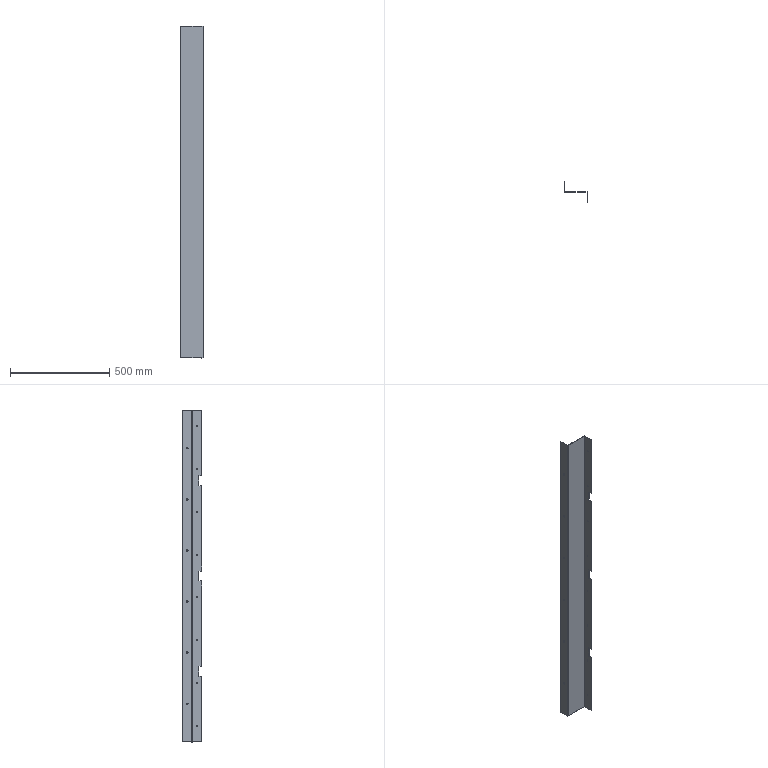Part | STEP file | TS-005-02 | 1 solid | 70 faces | box 120 x 98 x 1670 mm | volume 710619 mm3 | plane 38 | cylinder 32 | commonest cylinder face diameters 5.4 x16 8 x12 0.4 x2 4.4 x2